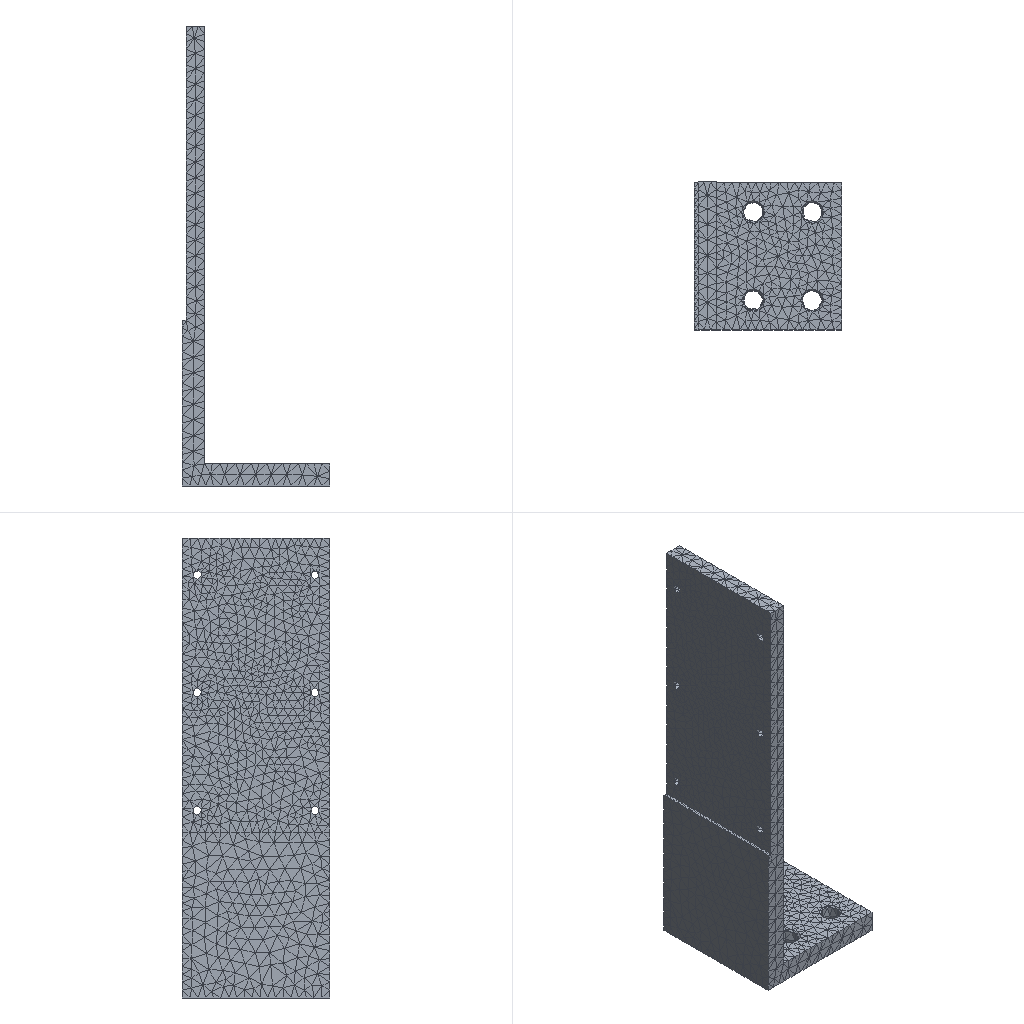Simulation study | ansys workbench
Set-up summary:
category,name,step,type,value,unit,region
solver,ansys_workbench
units,SI m-kg-s (Pa),,stated,"/units,MKS"
analysis,LS1,,static
load_step,LS1,LS1,static,nsubst=1; time=1
mesh,nodes,,,25089
mesh,elements,,,15549
element_type,SOLID187,,,14389
element_type,CONTA174,,,1160
material,Structural Steel,,E,2e+11,Pa
material,Structural Steel,,nu,0.3
material,Structural Steel,,density,7850,kg m^-3
material,Structural Steel,,conductivity,60.5,W m^-1 C^-1
material,Structural Steel,,specific_heat,434,J kg^-1 C^-1
material,Structural Steel,,cte,1.2e-05,C^-1
material,Structural Steel,,permeability,10000
material,Structural Steel,,resistivity,1.7e-07,kg m^3 A^-2 s^-3
load,,LS1,moment,"500 [dir=(1, 0, 0) n=3]",,all
bc,Fixed Supports,model,fixed,[dofs=ALL],,_FIXEDSU
contact,contact 1,,bonded (always),element=CONTA174
named_set,_FIXEDSU,,node,1125
Ansys APDL input file, long lists of numbers shortened:
/batch
/config,noeldb,1     ! force off writing results to database
*get,_wallstrt,active,,time,wall
! ANSYS input file written by Workbench version 2024 R1
! File used for geometry attach:
/title,wbnew--____ (A5)
! ****** Begin Custom Load Command Snippet ******
/COM, ACT Extensions:
/COM,     LSDYNA, 2024.1
/COM,/COM,     ANSYSMotion, 2024.1
/COM,
! ****** End   Custom Load Command Snippet ******
*DIM,_wb_ProjectScratch_dir,string,248
_wb_ProjectScratch_dir(1) = ''
*DIM,_wb_SolverFiles_dir,string,248
_wb_SolverFiles_dir(1) = ''
*DIM,_wb_userfiles_dir,string,248
_wb_userfiles_dir(1) = ''
/com,--- Data in consistent MKS units. See Solving Units in the help system for more information.
/units,MKS
/nopr
/wb,file,start              !  signify a WB generated input file
/prep7
! Turn off shape checking because checks already performed inside WB mesher.
! See help system for more information.
SHPP,OFF,,NOWARN
/nolist
etcon,set             ! allow ANSYS to choose best KEYOP's for 180x elements, resets any applicable keyopt to MAPDL defaults
/com,*********** Nodes for the whole assembly ***********
nblock,3,,27596
(1i9,3e20.9e3)
        1     1.000000000E-03     0.000000000E+00     1.250000000E-01
! (25087 more lines like these left out)
-1
/com,*********** Nodes for all Remote Points ***********
nblock,3
(1i9,3e20.9e3)
    25089     1.000000000E-03    -1.999999998E-02     8.501838191E-02
-1
/wb,elem,start            !  set before creation of elements
/com,*********** Elements for Body 1 "______" ***********
et,1,187
eblock,19,solid,,14389
(19i9)
        1        1        1        1        0        0        0        0       10        0        1     3626     3927     3909     3923    24795    25083    24793    24794
! (28777 more lines like these left out)
-1
/wb,elem,end               !  done creating elements
/com,*********** Send User Defined Coordinate System(s) ***********
csys,0
toffst,273.15,  ! Temperature offset from absolute zero
/com,*********** Set Reference Temperature ***********
tref,22.
/wb,mat,start              !  starting to send materials
/com,*********** Send Materials ***********
Temperature = 'TEMP' ! Temperature
MP,DENS,1,7850,	! kg m^-3
MP,ALPX,1,1.2e-05,	! C^-1
MP,C,1,434,	! J kg^-1 C^-1
MP,KXX,1,60.5,	! W m^-1 C^-1
MP,RSVX,1,1.7e-07,	! kg m^3 A^-2 s^-3
MP,EX,1,200000000000,	! Pa
MP,NUXY,1,0.3,
MP,MURX,1,10000,
/wb,mat,end                !  done sending materials
!************************* Model Summary ********************
!åéæ»å°åºåº§,	ç»æé¢,	matid,	1
!************************* End Model Summary ********************
! get the diagonal of the bounding box. Needed later for other things
*get,_xmin,node,,mnloc,x
*get,_ymin,node,,mnloc,y
*get,_zmin,node,,mnloc,z
*get,_xmax,node,,mxloc,x
*get,_ymax,node,,mxloc,y
*get,_zmax,node,,mxloc,z
_ASMDIAG=(_xmax-_xmin)*(_xmax-_xmin)+(_ymax-_ymin)*(_ymax-_ymin)+(_zmax-_zmin)*(_zmax-_zmin)
_ASMDIAG=SQRT(_ASMDIAG)
/wb,contact,start          !  starting to send contact
/wb,contact,end            !  done creating contacts
/golist
/wb,load,start             !  starting to send loads
/com,*********** Fixed Supports ***********
CMBLOCK,_FIXEDSU,NODE,     1125
(8i10)
       115       118       119       120       121       122       123       124
! (140 more lines like these left out)
cmsel,s,_FIXEDSU
d,all,all
nsel,all
/com,*********** Create Remote Point "ÄÚ²¿Ô¶³Ìµã" ***********
! -------- Remote Point Used by "Á¦¾Ø" --------
*set,tid,3
*set,cid,2
et,cid,174
et,tid,170
keyo,tid,2,1               ! Don't fix the pilot node
keyo,tid,4,111111
keyo,cid,12,5              ! Bonded Contact
keyo,cid,4,1               ! Deformable RBE3 style load
keyo,cid,2,2               ! MPC style contact
eblock,10,,,1160
(15i9)
    20043        2        2        2        0     1002     1213     1011     1011    10262    10339     1011    10260
! (1159 more lines like these left out)
-1
*set,_npilot,25089
_npilot31=_npilot
type,tid
mat ,cid
real,cid
tshape,pilo
en,21203,_npilot
tshape
/com,*********** Construct Moment Using Remote Attachment ***********
/gst,on,on
fini
*get,_numnode,node,0,count
*get,_numelem,elem,0,count
*get, _MAXELEMNUM, elem, 0, NUM, MAX
*get, _MAXNODENUM, node, 0, NUM, MAX
*get, _MAXELEMTYPE, etyp, 0, NUM, MAX
*get, _MAXREALCONST, rcon, 0, NUM, MAX
/go
/wb,load,end               !  done creating loads
/com,--- Number of total nodes = %_numnode%
/com,--- Number of contact elements = 1160
/com,--- Number of spring elements = 0
/com,--- Number of bearing elements = 0
/com,--- Number of solid elements = 14389
/com,--- Number of condensed parts = 0
/com,--- Number of total elements = %_numelem%
*get,_wallbsol,active,,time,wall
/com,****************************************************************************
/com,*************************    SOLUTION       ********************************
/com,****************************************************************************
/solu
antype,0                   ! static analysis
_thickRatio=  1     ! Ratio of thick parts in the model
eqsl,pcg,1e-8,,,,,,1
cntr,print,1               ! print out contact info and also make no initial contact an error
cncheck,dmp		!	Enable program controlled contact splitting for distributed memory parallel run
dmpoption,emat,no             ! Don't combine emat file for DANSYS
dmpoption,esav,no             ! Don't combine esav file for DANSYS
nldiag,cont,iter           ! print out contact info each equilibrium iteration
rescontrol,,none                 ! Do not keep any restart files
/com,****************************************************
/com,******************* SOLVE FOR LS 1 OF 1 ****************
nsel,s,node,,25089
f,all,mx,500.
f,all,my,0.
f,all,mz,0.
nsel,all
/nopr
/gopr
nsub,1,1,1
time,1.
outres,erase
outres,all,none
outres,nsol,all,
outres,rsol,all
outres,eangl,all
outres,etmp,all
outres,veng,all
outres,strs,all,
outres,epel,all,
outres,eppl,all,
outres,cont,all,
! *********** WB SOLVE COMMAND ***********
! check interactive state
*get,ANSINTER_,active,,int
*if,ANSINTER_,ne,0,then
/eof
*endif
solve
/com *************** Write FE CONNECTORS *********
CEWRITE,file,ce,,INTE
/com,****************************************************
/com,*************** FINISHED SOLVE FOR LS 1 *************
*get,_wallasol,active,,time,wall
/nopr
*get,_numnode,node,0,count
*get,_numelem,elem,0,count
*get, _MAXELEMNUM, elem, 0, NUM, MAX
*get, _MAXNODENUM, node, 0, NUM, MAX,,,INTERNAL
*get, _MAXELEMTYPE, etyp, 0, NUM, MAX
*get, _MAXREALCONST, rcon, 0, NUM, MAX
*get,_NSOLTHREADS,active,0,ntfs
*get,_NSOLPROCESSES,active,0,npfs
/gopr
*get,_PCGITER,active,,solu,cgiter
/post1
xmlo,ENCODING,ISO-8859-1
xmlo,parm
/xml,parm,xml
fini
/gopr
*get,_walldone,active,,time,wall
_preptime=(_wallbsol-_wallstrt)*3600
_solvtime=(_wallasol-_wallbsol)*3600
_posttime=(_walldone-_wallasol)*3600
_totaltim=(_walldone-_wallstrt)*3600
*get,_dlbratio,active,0,solu,dlbr
*get,_combtime,active,0,solu,comb
*get,_ssmode,active,0,solu,ssmm
*get,_ndofs,active,0,solu,ndof
*get,_sol_end_time,active,0,set,time
*if,_sol_end_time,eq,1.,then
/fclean				!clean distributed files
*endif
/com,--- Total number of nodes = %_numnode%
/com,--- Total number of elements = %_numelem%
/com,--- Element load balance ratio = %_dlbratio%
/com,--- Time to combine distributed files = %_combtime%
/com,--- Sparse memory mode = %_ssmode%
/com,--- Number of DOF = %_ndofs%
/wb,file,end               ! done with WB generated input
Results summary:
result,analyses[0].index,,,1
result,analyses[0].system,,,SYS
result,analyses[0].deck,,,deck.dat
result,analyses[0].solve_status,,,completed
result,analyses[0].analysis_type,,,static
result,analyses[0].physics,,,mechanical
result,analyses[0].unit_system,,,"MKS: m, kg, N, s, V, A, degC"
result,analyses[0].n_sets,,,1
result,analyses[0].load_steps[0].set,set=1,,1
result,analyses[0].load_steps[0].time_or_freq,set=1,,1
result,analyses[0].load_steps[0].max_displacement_magnitude,set=1,,0.0006586
result,analyses[0].load_steps[0].max_von_mises_nodal,set=1,,8.6878e+08
result,analyses[0].load_steps[0].reaction_force_sum_xyz[1],set=1,,8.64704e-06
result,analyses[0].load_steps[0].reaction_force_sum_xyz[2],set=1,,-4.13386e-05
result,analyses[0].load_steps[0].reaction_force_sum_xyz[3],set=1,,-1.63614e-08
result,geometry_export[0][0],,,.step
result,geometry_export[0][1],,,ok
result,geometry_export[0][2],,,1